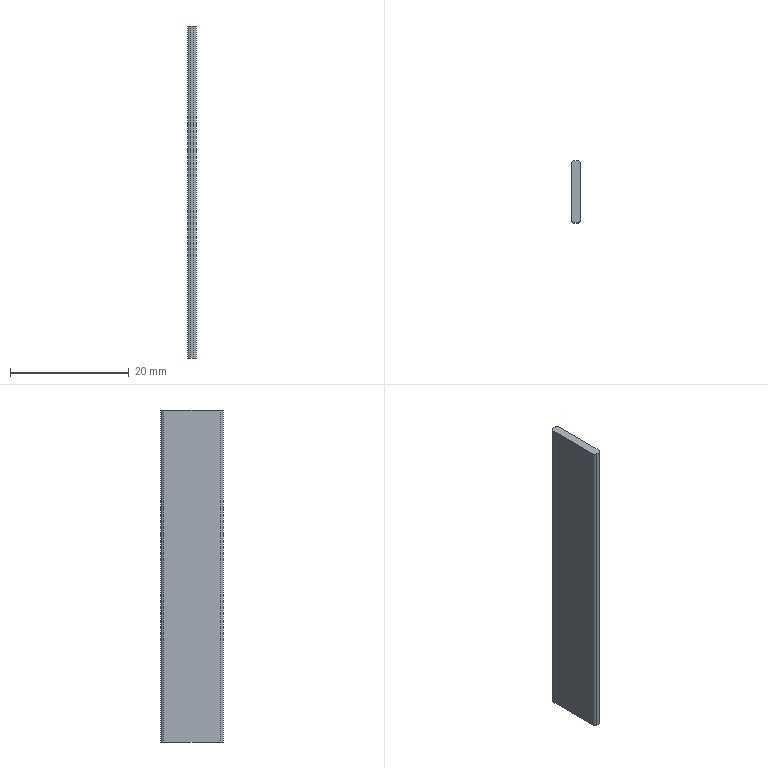Part | NX | features BREP 2 | 2 solids | 20 faces | box 1.5 x 10.5 x 56 mm | volume 1740 mm3 | plane 12 | cylinder 8 | commonest cylinder face diameters 1 x8
STEP:
#1=CARTESIAN_POINT('',(-0.25,5.25,-4.));
#2=VERTEX_POINT('',#1);
#3=CARTESIAN_POINT('',(-0.25,5.25,52.));
#4=VERTEX_POINT('',#3);
#5=CARTESIAN_POINT('',(-0.25,5.25,0.));
#6=DIRECTION('',(0.,0.,1.));
#7=VECTOR('',#6,1000.);
#8=LINE('',#5,#7);
#9=EDGE_CURVE('',#2,#4,#8,.T.);
#10=ORIENTED_EDGE('',*,*,#9,.T.);
#11=CARTESIAN_POINT('',(0.25,5.25,52.));
#12=VERTEX_POINT('',#11);
#13=CARTESIAN_POINT('',(-0.7765,5.25,52.));
#14=DIRECTION('',(-1.,0.,0.));
#15=VECTOR('',#14,1000.);
#16=LINE('',#13,#15);
#17=EDGE_CURVE('',#12,#4,#16,.T.);
#18=ORIENTED_EDGE('',*,*,#17,.F.);
#19=CARTESIAN_POINT('',(0.25,5.25,-4.));
#20=VERTEX_POINT('',#19);
#21=CARTESIAN_POINT('',(0.25,5.25,0.));
#22=DIRECTION('',(0.,0.,1.));
#23=VECTOR('',#22,1000.);
#24=LINE('',#21,#23);
#25=EDGE_CURVE('',#20,#12,#24,.T.);
#26=ORIENTED_EDGE('',*,*,#25,.F.);
#27=CARTESIAN_POINT('',(-0.7765,5.25,-4.));
#28=DIRECTION('',(-1.,0.,0.));
#29=VECTOR('',#28,1000.);
#30=LINE('',#27,#29);
#31=EDGE_CURVE('',#20,#2,#30,.T.);
#32=ORIENTED_EDGE('',*,*,#31,.T.);
#33=EDGE_LOOP('',(#10,#18,#26,#32));
#34=FACE_BOUND('',#33,.T.);
#35=CARTESIAN_POINT('',(0.25,5.25,0.));
#36=DIRECTION('',(0.,1.,0.));
#37=DIRECTION('',(1.,0.,0.));
#38=AXIS2_PLACEMENT_3D('',#35,#36,#37);
#39=PLANE('',#38);
#40=ADVANCED_FACE('',(#34),#39,.T.);
#41=ORIENTED_EDGE('',*,*,#25,.T.);
#42=CARTESIAN_POINT('',(0.75,4.75,52.));
#43=VERTEX_POINT('',#42);
#44=CARTESIAN_POINT('',(0.25,4.75,52.));
#45=DIRECTION('',(0.,0.,1.));
#46=DIRECTION('',(1.,0.,0.));
#47=AXIS2_PLACEMENT_3D('',#44,#45,#46);
#48=CIRCLE('',#47,0.5);
#49=EDGE_CURVE('',#43,#12,#48,.T.);
#50=ORIENTED_EDGE('',*,*,#49,.F.);
#51=CARTESIAN_POINT('',(0.75,4.75,-4.));
#52=VERTEX_POINT('',#51);
#53=CARTESIAN_POINT('',(0.75,4.75,0.));
#54=DIRECTION('',(0.,0.,1.));
#55=VECTOR('',#54,1000.);
#56=LINE('',#53,#55);
#57=EDGE_CURVE('',#52,#43,#56,.T.);
#58=ORIENTED_EDGE('',*,*,#57,.F.);
#59=CARTESIAN_POINT('',(0.25,4.75,-4.));
#60=DIRECTION('',(0.,0.,1.));
#61=DIRECTION('',(1.,0.,0.));
#62=AXIS2_PLACEMENT_3D('',#59,#60,#61);
#63=CIRCLE('',#62,0.5);
#64=EDGE_CURVE('',#52,#20,#63,.T.);
#65=ORIENTED_EDGE('',*,*,#64,.T.);
#66=EDGE_LOOP('',(#41,#50,#58,#65));
#67=FACE_BOUND('',#66,.T.);
#68=CARTESIAN_POINT('',(0.25,4.75,0.));
#69=DIRECTION('',(0.,0.,1.));
#70=DIRECTION('',(-1.,0.,0.));
#71=AXIS2_PLACEMENT_3D('',#68,#69,#70);
#72=CYLINDRICAL_SURFACE('',#71,0.5);
#73=ADVANCED_FACE('',(#67),#72,.T.);
#74=ORIENTED_EDGE('',*,*,#57,.T.);
#75=CARTESIAN_POINT('',(0.75,-4.75,52.));
#76=VERTEX_POINT('',#75);
#77=CARTESIAN_POINT('',(0.75,4.728,52.));
#78=DIRECTION('',(0.,1.,0.));
#79=VECTOR('',#78,1000.);
#80=LINE('',#77,#79);
#81=EDGE_CURVE('',#76,#43,#80,.T.);
#82=ORIENTED_EDGE('',*,*,#81,.F.);
#83=CARTESIAN_POINT('',(0.75,-4.75,-4.));
#84=VERTEX_POINT('',#83);
#85=CARTESIAN_POINT('',(0.75,-4.75,0.));
#86=DIRECTION('',(0.,0.,1.));
#87=VECTOR('',#86,1000.);
#88=LINE('',#85,#87);
#89=EDGE_CURVE('',#84,#76,#88,.T.);
#90=ORIENTED_EDGE('',*,*,#89,.F.);
#91=CARTESIAN_POINT('',(0.75,4.728,-4.));
#92=DIRECTION('',(0.,1.,0.));
#93=VECTOR('',#92,1000.);
#94=LINE('',#91,#93);
#95=EDGE_CURVE('',#84,#52,#94,.T.);
#96=ORIENTED_EDGE('',*,*,#95,.T.);
#97=EDGE_LOOP('',(#74,#82,#90,#96));
#98=FACE_BOUND('',#97,.T.);
#99=CARTESIAN_POINT('',(0.75,-4.75,0.));
#100=DIRECTION('',(1.,0.,0.));
#101=DIRECTION('',(0.,-1.,0.));
#102=AXIS2_PLACEMENT_3D('',#99,#100,#101);
#103=PLANE('',#102);
#104=ADVANCED_FACE('',(#98),#103,.T.);
#105=ORIENTED_EDGE('',*,*,#89,.T.);
#106=CARTESIAN_POINT('',(0.25,-5.25,52.));
#107=VERTEX_POINT('',#106);
#108=CARTESIAN_POINT('',(0.25,-4.75,52.));
#109=DIRECTION('',(0.,0.,1.));
#110=DIRECTION('',(1.,0.,0.));
#111=AXIS2_PLACEMENT_3D('',#108,#109,#110);
#112=CIRCLE('',#111,0.5);
#113=EDGE_CURVE('',#107,#76,#112,.T.);
#114=ORIENTED_EDGE('',*,*,#113,.F.);
#115=CARTESIAN_POINT('',(0.25,-5.25,-4.));
#116=VERTEX_POINT('',#115);
#117=CARTESIAN_POINT('',(0.25,-5.25,0.));
#118=DIRECTION('',(0.,0.,1.));
#119=VECTOR('',#118,1000.);
#120=LINE('',#117,#119);
#121=EDGE_CURVE('',#116,#107,#120,.T.);
#122=ORIENTED_EDGE('',*,*,#121,.F.);
#123=CARTESIAN_POINT('',(0.25,-4.75,-4.));
#124=DIRECTION('',(0.,0.,1.));
#125=DIRECTION('',(1.,0.,0.));
#126=AXIS2_PLACEMENT_3D('',#123,#124,#125);
#127=CIRCLE('',#126,0.5);
#128=EDGE_CURVE('',#116,#84,#127,.T.);
#129=ORIENTED_EDGE('',*,*,#128,.T.);
#130=EDGE_LOOP('',(#105,#114,#122,#129));
#131=FACE_BOUND('',#130,.T.);
#132=CARTESIAN_POINT('',(0.25,-4.75,0.));
#133=DIRECTION('',(0.,0.,1.));
#134=DIRECTION('',(-1.,0.,0.));
#135=AXIS2_PLACEMENT_3D('',#132,#133,#134);
#136=CYLINDRICAL_SURFACE('',#135,0.5);
#137=ADVANCED_FACE('',(#131),#136,.T.);
#138=ORIENTED_EDGE('',*,*,#121,.T.);
#139=CARTESIAN_POINT('',(-0.25,-5.25,52.));
#140=VERTEX_POINT('',#139);
#141=CARTESIAN_POINT('',(-0.7765,-5.25,52.));
#142=DIRECTION('',(1.,0.,0.));
#143=VECTOR('',#142,1000.);
#144=LINE('',#141,#143);
#145=EDGE_CURVE('',#140,#107,#144,.T.);
#146=ORIENTED_EDGE('',*,*,#145,.F.);
#147=CARTESIAN_POINT('',(-0.25,-5.25,-4.));
#148=VERTEX_POINT('',#147);
#149=CARTESIAN_POINT('',(-0.25,-5.25,0.));
#150=DIRECTION('',(0.,0.,1.));
#151=VECTOR('',#150,1000.);
#152=LINE('',#149,#151);
#153=EDGE_CURVE('',#148,#140,#152,.T.);
#154=ORIENTED_EDGE('',*,*,#153,.F.);
#155=CARTESIAN_POINT('',(-0.7765,-5.25,-4.));
#156=DIRECTION('',(1.,0.,0.));
#157=VECTOR('',#156,1000.);
#158=LINE('',#155,#157);
#159=EDGE_CURVE('',#148,#116,#158,.T.);
#160=ORIENTED_EDGE('',*,*,#159,.T.);
#161=EDGE_LOOP('',(#138,#146,#154,#160));
#162=FACE_BOUND('',#161,.T.);
#163=CARTESIAN_POINT('',(-0.25,-5.25,0.));
#164=DIRECTION('',(0.,-1.,0.));
#165=DIRECTION('',(-1.,0.,0.));
#166=AXIS2_PLACEMENT_3D('',#163,#164,#165);
#167=PLANE('',#166);
#168=ADVANCED_FACE('',(#162),#167,.T.);
#169=ORIENTED_EDGE('',*,*,#153,.T.);
#170=CARTESIAN_POINT('',(-0.75,-4.75,52.));
#171=VERTEX_POINT('',#170);
#172=CARTESIAN_POINT('',(-0.25,-4.75,52.));
#173=DIRECTION('',(0.,0.,1.));
#174=DIRECTION('',(1.,0.,0.));
#175=AXIS2_PLACEMENT_3D('',#172,#173,#174);
#176=CIRCLE('',#175,0.5);
#177=EDGE_CURVE('',#171,#140,#176,.T.);
#178=ORIENTED_EDGE('',*,*,#177,.F.);
#179=CARTESIAN_POINT('',(-0.75,-4.75,-4.));
#180=VERTEX_POINT('',#179);
#181=CARTESIAN_POINT('',(-0.75,-4.75,0.));
#182=DIRECTION('',(0.,0.,1.));
#183=VECTOR('',#182,1000.);
#184=LINE('',#181,#183);
#185=EDGE_CURVE('',#180,#171,#184,.T.);
#186=ORIENTED_EDGE('',*,*,#185,.F.);
#187=CARTESIAN_POINT('',(-0.25,-4.75,-4.));
#188=DIRECTION('',(0.,0.,1.));
#189=DIRECTION('',(1.,0.,0.));
#190=AXIS2_PLACEMENT_3D('',#187,#188,#189);
#191=CIRCLE('',#190,0.5);
#192=EDGE_CURVE('',#180,#148,#191,.T.);
#193=ORIENTED_EDGE('',*,*,#192,.T.);
#194=EDGE_LOOP('',(#169,#178,#186,#193));
#195=FACE_BOUND('',#194,.T.);
#196=CARTESIAN_POINT('',(-0.25,-4.75,0.));
#197=DIRECTION('',(0.,0.,1.));
#198=DIRECTION('',(-1.,0.,0.));
#199=AXIS2_PLACEMENT_3D('',#196,#197,#198);
#200=CYLINDRICAL_SURFACE('',#199,0.5);
#201=ADVANCED_FACE('',(#195),#200,.T.);
#202=ORIENTED_EDGE('',*,*,#185,.T.);
#203=CARTESIAN_POINT('',(-0.75,4.75,52.));
#204=VERTEX_POINT('',#203);
#205=CARTESIAN_POINT('',(-0.75,4.728,52.));
#206=DIRECTION('',(0.,-1.,0.));
#207=VECTOR('',#206,1000.);
#208=LINE('',#205,#207);
#209=EDGE_CURVE('',#204,#171,#208,.T.);
#210=ORIENTED_EDGE('',*,*,#209,.F.);
#211=CARTESIAN_POINT('',(-0.75,4.75,-4.));
#212=VERTEX_POINT('',#211);
#213=CARTESIAN_POINT('',(-0.75,4.75,0.));
#214=DIRECTION('',(0.,0.,1.));
#215=VECTOR('',#214,1000.);
#216=LINE('',#213,#215);
#217=EDGE_CURVE('',#212,#204,#216,.T.);
#218=ORIENTED_EDGE('',*,*,#217,.F.);
#219=CARTESIAN_POINT('',(-0.75,4.728,-4.));
#220=DIRECTION('',(0.,-1.,0.));
#221=VECTOR('',#220,1000.);
#222=LINE('',#219,#221);
#223=EDGE_CURVE('',#212,#180,#222,.T.);
#224=ORIENTED_EDGE('',*,*,#223,.T.);
#225=EDGE_LOOP('',(#202,#210,#218,#224));
#226=FACE_BOUND('',#225,.T.);
#227=CARTESIAN_POINT('',(-0.75,4.75,0.));
#228=DIRECTION('',(-1.,0.,0.));
#229=DIRECTION('',(0.,1.,0.));
#230=AXIS2_PLACEMENT_3D('',#227,#228,#229);
#231=PLANE('',#230);
#232=ADVANCED_FACE('',(#226),#231,.T.);
#233=CARTESIAN_POINT('',(-0.25,4.75,-4.));
#234=DIRECTION('',(0.,0.,1.));
#235=DIRECTION('',(1.,0.,0.));
#236=AXIS2_PLACEMENT_3D('',#233,#234,#235);
#237=CIRCLE('',#236,0.5);
#238=EDGE_CURVE('',#2,#212,#237,.T.);
#239=ORIENTED_EDGE('',*,*,#238,.T.);
#240=ORIENTED_EDGE('',*,*,#217,.T.);
#241=CARTESIAN_POINT('',(-0.25,4.75,52.));
#242=DIRECTION('',(0.,0.,1.));
#243=DIRECTION('',(1.,0.,0.));
#244=AXIS2_PLACEMENT_3D('',#241,#242,#243);
#245=CIRCLE('',#244,0.5);
#246=EDGE_CURVE('',#4,#204,#245,.T.);
#247=ORIENTED_EDGE('',*,*,#246,.F.);
#248=ORIENTED_EDGE('',*,*,#9,.F.);
#249=EDGE_LOOP('',(#239,#240,#247,#248));
#250=FACE_BOUND('',#249,.T.);
#251=CARTESIAN_POINT('',(-0.25,4.75,0.));
#252=DIRECTION('',(0.,0.,1.));
#253=DIRECTION('',(-1.,0.,0.));
#254=AXIS2_PLACEMENT_3D('',#251,#252,#253);
#255=CYLINDRICAL_SURFACE('',#254,0.5);
#256=ADVANCED_FACE('',(#250),#255,.T.);
#257=ORIENTED_EDGE('',*,*,#209,.T.);
#258=ORIENTED_EDGE('',*,*,#177,.T.);
#259=ORIENTED_EDGE('',*,*,#145,.T.);
#260=ORIENTED_EDGE('',*,*,#113,.T.);
#261=ORIENTED_EDGE('',*,*,#81,.T.);
#262=ORIENTED_EDGE('',*,*,#49,.T.);
#263=ORIENTED_EDGE('',*,*,#17,.T.);
#264=ORIENTED_EDGE('',*,*,#246,.T.);
#265=EDGE_LOOP('',(#257,#258,#259,#260,#261,#262,#263,#264));
#266=FACE_BOUND('',#265,.T.);
#267=CARTESIAN_POINT('',(-0.7765,4.728,52.));
#268=DIRECTION('',(0.,0.,1.));
#269=DIRECTION('',(-1.,0.,0.));
#270=AXIS2_PLACEMENT_3D('',#267,#268,#269);
#271=PLANE('',#270);
#272=ADVANCED_FACE('',(#266),#271,.T.);
#273=ORIENTED_EDGE('',*,*,#223,.F.);
#274=ORIENTED_EDGE('',*,*,#238,.F.);
#275=ORIENTED_EDGE('',*,*,#31,.F.);
#276=ORIENTED_EDGE('',*,*,#64,.F.);
#277=ORIENTED_EDGE('',*,*,#95,.F.);
#278=ORIENTED_EDGE('',*,*,#128,.F.);
#279=ORIENTED_EDGE('',*,*,#159,.F.);
#280=ORIENTED_EDGE('',*,*,#192,.F.);
#281=EDGE_LOOP('',(#273,#274,#275,#276,#277,#278,#279,#280));
#282=FACE_BOUND('',#281,.T.);
#283=CARTESIAN_POINT('',(-0.7765,4.728,-4.));
#284=DIRECTION('',(0.,0.,1.));
#285=DIRECTION('',(-1.,0.,0.));
#286=AXIS2_PLACEMENT_3D('',#283,#284,#285);
#287=PLANE('',#286);
#288=ADVANCED_FACE('',(#282),#287,.F.);
#289=CLOSED_SHELL('',(#40,#73,#104,#137,#168,#201,#232,#256,#272,#288));
#290=MANIFOLD_SOLID_BREP('',#289);
#291=CARTESIAN_POINT('',(-0.25,5.25,-4.));
#292=VERTEX_POINT('',#291);
#293=CARTESIAN_POINT('',(-0.25,5.25,52.));
#294=VERTEX_POINT('',#293);
#295=CARTESIAN_POINT('',(-0.25,5.25,0.));
#296=DIRECTION('',(0.,0.,1.));
#297=VECTOR('',#296,1000.);
#298=LINE('',#295,#297);
#299=EDGE_CURVE('',#292,#294,#298,.T.);
#300=ORIENTED_EDGE('',*,*,#299,.T.);
#301=CARTESIAN_POINT('',(0.25,5.25,52.));
#302=VERTEX_POINT('',#301);
#303=CARTESIAN_POINT('',(-0.7765,5.25,52.));
#304=DIRECTION('',(-1.,0.,0.));
#305=VECTOR('',#304,1000.);
#306=LINE('',#303,#305);
#307=EDGE_CURVE('',#302,#294,#306,.T.);
#308=ORIENTED_EDGE('',*,*,#307,.F.);
#309=CARTESIAN_POINT('',(0.25,5.25,-4.));
#310=VERTEX_POINT('',#309);
#311=CARTESIAN_POINT('',(0.25,5.25,0.));
#312=DIRECTION('',(0.,0.,1.));
#313=VECTOR('',#312,1000.);
#314=LINE('',#311,#313);
#315=EDGE_CURVE('',#310,#302,#314,.T.);
#316=ORIENTED_EDGE('',*,*,#315,.F.);
#317=CARTESIAN_POINT('',(-0.7765,5.25,-4.));
#318=DIRECTION('',(-1.,0.,0.));
#319=VECTOR('',#318,1000.);
#320=LINE('',#317,#319);
#321=EDGE_CURVE('',#310,#292,#320,.T.);
#322=ORIENTED_EDGE('',*,*,#321,.T.);
#323=EDGE_LOOP('',(#300,#308,#316,#322));
#324=FACE_BOUND('',#323,.T.);
#325=CARTESIAN_POINT('',(0.25,5.25,0.));
#326=DIRECTION('',(0.,1.,0.));
#327=DIRECTION('',(1.,0.,0.));
#328=AXIS2_PLACEMENT_3D('',#325,#326,#327);
#329=PLANE('',#328);
#330=ADVANCED_FACE('',(#324),#329,.T.);
#331=ORIENTED_EDGE('',*,*,#315,.T.);
#332=CARTESIAN_POINT('',(0.75,4.75,52.));
#333=VERTEX_POINT('',#332);
#334=CARTESIAN_POINT('',(0.25,4.75,52.));
#335=DIRECTION('',(0.,0.,1.));
#336=DIRECTION('',(1.,0.,0.));
#337=AXIS2_PLACEMENT_3D('',#334,#335,#336);
#338=CIRCLE('',#337,0.5);
#339=EDGE_CURVE('',#333,#302,#338,.T.);
#340=ORIENTED_EDGE('',*,*,#339,.F.);
#341=CARTESIAN_POINT('',(0.75,4.75,-4.));
#342=VERTEX_POINT('',#341);
#343=CARTESIAN_POINT('',(0.75,4.75,0.));
#344=DIRECTION('',(0.,0.,1.));
#345=VECTOR('',#344,1000.);
#346=LINE('',#343,#345);
#347=EDGE_CURVE('',#342,#333,#346,.T.);
#348=ORIENTED_EDGE('',*,*,#347,.F.);
#349=CARTESIAN_POINT('',(0.25,4.75,-4.));
#350=DIRECTION('',(0.,0.,1.));
#351=DIRECTION('',(1.,0.,0.));
#352=AXIS2_PLACEMENT_3D('',#349,#350,#351);
#353=CIRCLE('',#352,0.5);
#354=EDGE_CURVE('',#342,#310,#353,.T.);
#355=ORIENTED_EDGE('',*,*,#354,.T.);
#356=EDGE_LOOP('',(#331,#340,#348,#355));
#357=FACE_BOUND('',#356,.T.);
#358=CARTESIAN_POINT('',(0.25,4.75,0.));
#359=DIRECTION('',(0.,0.,1.));
#360=DIRECTION('',(-1.,0.,0.));
#361=AXIS2_PLACEMENT_3D('',#358,#359,#360);
#362=CYLINDRICAL_SURFACE('',#361,0.5);
#363=ADVANCED_FACE('',(#357),#362,.T.);
#364=ORIENTED_EDGE('',*,*,#347,.T.);
#365=CARTESIAN_POINT('',(0.75,-4.75,52.));
#366=VERTEX_POINT('',#365);
#367=CARTESIAN_POINT('',(0.75,4.728,52.));
#368=DIRECTION('',(0.,1.,0.));
#369=VECTOR('',#368,1000.);
#370=LINE('',#367,#369);
#371=EDGE_CURVE('',#366,#333,#370,.T.);
#372=ORIENTED_EDGE('',*,*,#371,.F.);
#373=CARTESIAN_POINT('',(0.75,-4.75,-4.));
#374=VERTEX_POINT('',#373);
#375=CARTESIAN_POINT('',(0.75,-4.75,0.));
#376=DIRECTION('',(0.,0.,1.));
#377=VECTOR('',#376,1000.);
#378=LINE('',#375,#377);
#379=EDGE_CURVE('',#374,#366,#378,.T.);
#380=ORIENTED_EDGE('',*,*,#379,.F.);
#381=CARTESIAN_POINT('',(0.75,4.728,-4.));
#382=DIRECTION('',(0.,1.,0.));
#383=VECTOR('',#382,1000.);
#384=LINE('',#381,#383);
#385=EDGE_CURVE('',#374,#342,#384,.T.);
#386=ORIENTED_EDGE('',*,*,#385,.T.);
#387=EDGE_LOOP('',(#364,#372,#380,#386));
#388=FACE_BOUND('',#387,.T.);
#389=CARTESIAN_POINT('',(0.75,-4.75,0.));
#390=DIRECTION('',(1.,0.,0.));
#391=DIRECTION('',(0.,-1.,0.));
#392=AXIS2_PLACEMENT_3D('',#389,#390,#391);
#393=PLANE('',#392);
#394=ADVANCED_FACE('',(#388),#393,.T.);
#395=ORIENTED_EDGE('',*,*,#379,.T.);
#396=CARTESIAN_POINT('',(0.25,-5.25,52.));
#397=VERTEX_POINT('',#396);
#398=CARTESIAN_POINT('',(0.25,-4.75,52.));
#399=DIRECTION('',(0.,0.,1.));
#400=DIRECTION('',(1.,0.,0.));
#401=AXIS2_PLACEMENT_3D('',#398,#399,#400);
#402=CIRCLE('',#401,0.5);
#403=EDGE_CURVE('',#397,#366,#402,.T.);
#404=ORIENTED_EDGE('',*,*,#403,.F.);
#405=CARTESIAN_POINT('',(0.25,-5.25,-4.));
#406=VERTEX_POINT('',#405);
#407=CARTESIAN_POINT('',(0.25,-5.25,0.));
#408=DIRECTION('',(0.,0.,1.));
#409=VECTOR('',#408,1000.);
#410=LINE('',#407,#409);
#411=EDGE_CURVE('',#406,#397,#410,.T.);
#412=ORIENTED_EDGE('',*,*,#411,.F.);
#413=CARTESIAN_POINT('',(0.25,-4.75,-4.));
#414=DIRECTION('',(0.,0.,1.));
#415=DIRECTION('',(1.,0.,0.));
#416=AXIS2_PLACEMENT_3D('',#413,#414,#415);
#417=CIRCLE('',#416,0.5);
#418=EDGE_CURVE('',#406,#374,#417,.T.);
#419=ORIENTED_EDGE('',*,*,#418,.T.);
#420=EDGE_LOOP('',(#395,#404,#412,#419));
#421=FACE_BOUND('',#420,.T.);
#422=CARTESIAN_POINT('',(0.25,-4.75,0.));
#423=DIRECTION('',(0.,0.,1.));
#424=DIRECTION('',(-1.,0.,0.));
#425=AXIS2_PLACEMENT_3D('',#422,#423,#424);
#426=CYLINDRICAL_SURFACE('',#425,0.5);
#427=ADVANCED_FACE('',(#421),#426,.T.);
#428=ORIENTED_EDGE('',*,*,#411,.T.);
#429=CARTESIAN_POINT('',(-0.25,-5.25,52.));
#430=VERTEX_POINT('',#429);
#431=CARTESIAN_POINT('',(-0.7765,-5.25,52.));
#432=DIRECTION('',(1.,0.,0.));
#433=VECTOR('',#432,1000.);
#434=LINE('',#431,#433);
#435=EDGE_CURVE('',#430,#397,#434,.T.);
#436=ORIENTED_EDGE('',*,*,#435,.F.);
#437=CARTESIAN_POINT('',(-0.25,-5.25,-4.));
#438=VERTEX_POINT('',#437);
#439=CARTESIAN_POINT('',(-0.25,-5.25,0.));
#440=DIRECTION('',(0.,0.,1.));
#441=VECTOR('',#440,1000.);
#442=LINE('',#439,#441);
#443=EDGE_CURVE('',#438,#430,#442,.T.);
#444=ORIENTED_EDGE('',*,*,#443,.F.);
#445=CARTESIAN_POINT('',(-0.7765,-5.25,-4.));
#446=DIRECTION('',(1.,0.,0.));
#447=VECTOR('',#446,1000.);
#448=LINE('',#445,#447);
#449=EDGE_CURVE('',#438,#406,#448,.T.);
#450=ORIENTED_EDGE('',*,*,#449,.T.);
#451=EDGE_LOOP('',(#428,#436,#444,#450));
#452=FACE_BOUND('',#451,.T.);
#453=CARTESIAN_POINT('',(-0.25,-5.25,0.));
#454=DIRECTION('',(0.,-1.,0.));
#455=DIRECTION('',(-1.,0.,0.));
#456=AXIS2_PLACEMENT_3D('',#453,#454,#455);
#457=PLANE('',#456);
#458=ADVANCED_FACE('',(#452),#457,.T.);
#459=ORIENTED_EDGE('',*,*,#443,.T.);
#460=CARTESIAN_POINT('',(-0.75,-4.75,52.));
#461=VERTEX_POINT('',#460);
#462=CARTESIAN_POINT('',(-0.25,-4.75,52.));
#463=DIRECTION('',(0.,0.,1.));
#464=DIRECTION('',(1.,0.,0.));
#465=AXIS2_PLACEMENT_3D('',#462,#463,#464);
#466=CIRCLE('',#465,0.5);
#467=EDGE_CURVE('',#461,#430,#466,.T.);
#468=ORIENTED_EDGE('',*,*,#467,.F.);
#469=CARTESIAN_POINT('',(-0.75,-4.75,-4.));
#470=VERTEX_POINT('',#469);
#471=CARTESIAN_POINT('',(-0.75,-4.75,0.));
#472=DIRECTION('',(0.,0.,1.));
#473=VECTOR('',#472,1000.);
#474=LINE('',#471,#473);
#475=EDGE_CURVE('',#470,#461,#474,.T.);
#476=ORIENTED_EDGE('',*,*,#475,.F.);
#477=CARTESIAN_POINT('',(-0.25,-4.75,-4.));
#478=DIRECTION('',(0.,0.,1.));
#479=DIRECTION('',(1.,0.,0.));
#480=AXIS2_PLACEMENT_3D('',#477,#478,#479);
#481=CIRCLE('',#480,0.5);
#482=EDGE_CURVE('',#470,#438,#481,.T.);
#483=ORIENTED_EDGE('',*,*,#482,.T.);
#484=EDGE_LOOP('',(#459,#468,#476,#483));
#485=FACE_BOUND('',#484,.T.);
#486=CARTESIAN_POINT('',(-0.25,-4.75,0.));
#487=DIRECTION('',(0.,0.,1.));
#488=DIRECTION('',(-1.,0.,0.));
#489=AXIS2_PLACEMENT_3D('',#486,#487,#488);
#490=CYLINDRICAL_SURFACE('',#489,0.5);
#491=ADVANCED_FACE('',(#485),#490,.T.);
#492=ORIENTED_EDGE('',*,*,#475,.T.);
#493=CARTESIAN_POINT('',(-0.75,4.75,52.));
#494=VERTEX_POINT('',#493);
#495=CARTESIAN_POINT('',(-0.75,4.728,52.));
#496=DIRECTION('',(0.,-1.,0.));
#497=VECTOR('',#496,1000.);
#498=LINE('',#495,#497);
#499=EDGE_CURVE('',#494,#461,#498,.T.);
#500=ORIENTED_EDGE('',*,*,#499,.F.);
#501=CARTESIAN_POINT('',(-0.75,4.75,-4.));
#502=VERTEX_POINT('',#501);
#503=CARTESIAN_POINT('',(-0.75,4.75,0.));
#504=DIRECTION('',(0.,0.,1.));
#505=VECTOR('',#504,1000.);
#506=LINE('',#503,#505);
#507=EDGE_CURVE('',#502,#494,#506,.T.);
#508=ORIENTED_EDGE('',*,*,#507,.F.);
#509=CARTESIAN_POINT('',(-0.75,4.728,-4.));
#510=DIRECTION('',(0.,-1.,0.));
#511=VECTOR('',#510,1000.);
#512=LINE('',#509,#511);
#513=EDGE_CURVE('',#502,#470,#512,.T.);
#514=ORIENTED_EDGE('',*,*,#513,.T.);
#515=EDGE_LOOP('',(#492,#500,#508,#514));
#516=FACE_BOUND('',#515,.T.);
#517=CARTESIAN_POINT('',(-0.75,4.75,0.));
#518=DIRECTION('',(-1.,0.,0.));
#519=DIRECTION('',(0.,1.,0.));
#520=AXIS2_PLACEMENT_3D('',#517,#518,#519);
#521=PLANE('',#520);
#522=ADVANCED_FACE('',(#516),#521,.T.);
#523=CARTESIAN_POINT('',(-0.25,4.75,-4.));
#524=DIRECTION('',(0.,0.,1.));
#525=DIRECTION('',(1.,0.,0.));
#526=AXIS2_PLACEMENT_3D('',#523,#524,#525);
#527=CIRCLE('',#526,0.5);
#528=EDGE_CURVE('',#292,#502,#527,.T.);
#529=ORIENTED_EDGE('',*,*,#528,.T.);
#530=ORIENTED_EDGE('',*,*,#507,.T.);
#531=CARTESIAN_POINT('',(-0.25,4.75,52.));
#532=DIRECTION('',(0.,0.,1.));
#533=DIRECTION('',(1.,0.,0.));
#534=AXIS2_PLACEMENT_3D('',#531,#532,#533);
#535=CIRCLE('',#534,0.5);
#536=EDGE_CURVE('',#294,#494,#535,.T.);
#537=ORIENTED_EDGE('',*,*,#536,.F.);
#538=ORIENTED_EDGE('',*,*,#299,.F.);
#539=EDGE_LOOP('',(#529,#530,#537,#538));
#540=FACE_BOUND('',#539,.T.);
#541=CARTESIAN_POINT('',(-0.25,4.75,0.));
#542=DIRECTION('',(0.,0.,1.));
#543=DIRECTION('',(-1.,0.,0.));
#544=AXIS2_PLACEMENT_3D('',#541,#542,#543);
#545=CYLINDRICAL_SURFACE('',#544,0.5);
#546=ADVANCED_FACE('',(#540),#545,.T.);
#547=ORIENTED_EDGE('',*,*,#499,.T.);
#548=ORIENTED_EDGE('',*,*,#467,.T.);
#549=ORIENTED_EDGE('',*,*,#435,.T.);
#550=ORIENTED_EDGE('',*,*,#403,.T.);
#551=ORIENTED_EDGE('',*,*,#371,.T.);
#552=ORIENTED_EDGE('',*,*,#339,.T.);
#553=ORIENTED_EDGE('',*,*,#307,.T.);
#554=ORIENTED_EDGE('',*,*,#536,.T.);
#555=EDGE_LOOP('',(#547,#548,#549,#550,#551,#552,#553,#554));
#556=FACE_BOUND('',#555,.T.);
#557=CARTESIAN_POINT('',(-0.7765,4.728,52.));
#558=DIRECTION('',(0.,0.,1.));
#559=DIRECTION('',(-1.,0.,0.));
#560=AXIS2_PLACEMENT_3D('',#557,#558,#559);
#561=PLANE('',#560);
#562=ADVANCED_FACE('',(#556),#561,.T.);
#563=ORIENTED_EDGE('',*,*,#513,.F.);
#564=ORIENTED_EDGE('',*,*,#528,.F.);
#565=ORIENTED_EDGE('',*,*,#321,.F.);
#566=ORIENTED_EDGE('',*,*,#354,.F.);
#567=ORIENTED_EDGE('',*,*,#385,.F.);
#568=ORIENTED_EDGE('',*,*,#418,.F.);
#569=ORIENTED_EDGE('',*,*,#449,.F.);
#570=ORIENTED_EDGE('',*,*,#482,.F.);
#571=EDGE_LOOP('',(#563,#564,#565,#566,#567,#568,#569,#570));
#572=FACE_BOUND('',#571,.T.);
#573=CARTESIAN_POINT('',(-0.7765,4.728,-4.));
#574=DIRECTION('',(0.,0.,1.));
#575=DIRECTION('',(-1.,0.,0.));
#576=AXIS2_PLACEMENT_3D('',#573,#574,#575);
#577=PLANE('',#576);
#578=ADVANCED_FACE('',(#572),#577,.F.);
#579=CLOSED_SHELL('',(#330,#363,#394,#427,#458,#491,#522,#546,#562,#578));
#580=MANIFOLD_SOLID_BREP('',#579);
#581=(LENGTH_UNIT()NAMED_UNIT(*)SI_UNIT(.MILLI.,.METRE.));
#582=UNCERTAINTY_MEASURE_WITH_UNIT(LENGTH_MEASURE(0.00001),#581,'','');
#583=(NAMED_UNIT(*)PLANE_ANGLE_UNIT()SI_UNIT($,.RADIAN.));
#584=(NAMED_UNIT(*)SI_UNIT($,.STERADIAN.)SOLID_ANGLE_UNIT());
#585=(GEOMETRIC_REPRESENTATION_CONTEXT(3)GLOBAL_UNCERTAINTY_ASSIGNED_CONTEXT((#582))GLOBAL_UNIT_ASSIGNED_CONTEXT((#581,#583,#584))REPRESENTATION_CONTEXT('',''));
#586=ADVANCED_BREP_SHAPE_REPRESENTATION('',(#290,#580),#585);